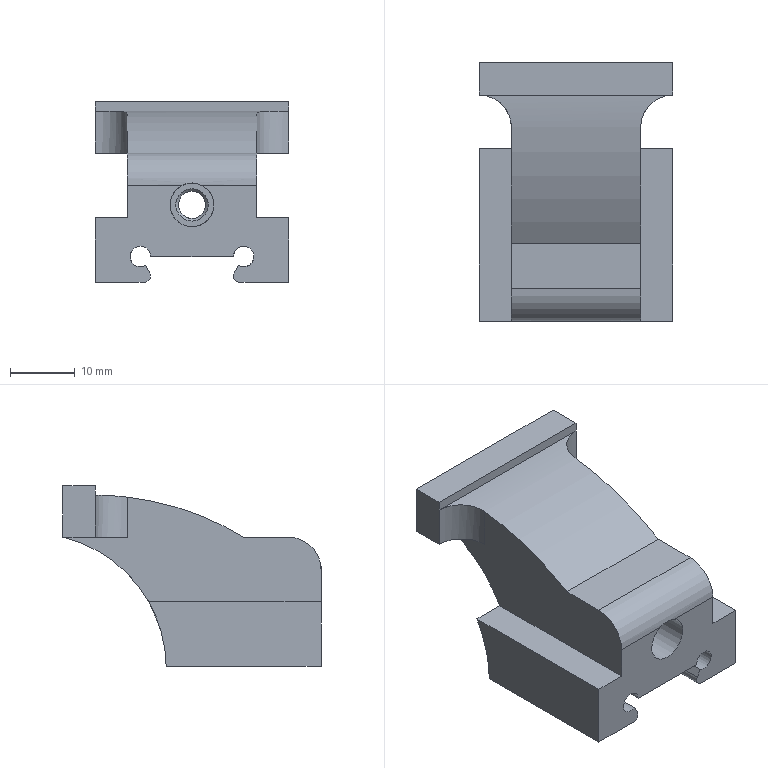Part | NX | features SKETCH 9, EXTRUDE 8, BLEND 3, DATUM_CSYS 1, HOLE PACKAGE 1, SIMPLE HOLE 1, SYMBOLIC_THREAD 1 | 1 solid | 34 faces | box 30 x 40 x 28 mm | volume 14530 mm3 | plane 21 | cylinder 11 | cone 1 | spline 1 | commonest cylinder face diameters 10 x3 2 x2 3.2 x2 4.2 x1 6.8 x1 41.718 x1
STEP:
#1=CARTESIAN_POINT('',(-7.423,0.,-12.));
#2=VERTEX_POINT('',#1);
#3=CARTESIAN_POINT('',(-15.,0.,-12.));
#4=VERTEX_POINT('',#3);
#5=CARTESIAN_POINT('',(15.,0.,-12.));
#6=DIRECTION('',(-1.,0.,0.));
#7=VECTOR('',#6,1000.);
#8=LINE('',#5,#7);
#9=EDGE_CURVE('',#2,#4,#8,.T.);
#10=ORIENTED_EDGE('',*,*,#9,.F.);
#11=CARTESIAN_POINT('',(-6.557,0.,-10.5));
#12=VERTEX_POINT('',#11);
#13=CARTESIAN_POINT('',(-7.423,0.,-11.));
#14=DIRECTION('',(0.,1.,0.));
#15=DIRECTION('',(0.,0.,1.));
#16=AXIS2_PLACEMENT_3D('',#13,#14,#15);
#17=CIRCLE('',#16,1.);
#18=EDGE_CURVE('',#2,#12,#17,.F.);
#19=ORIENTED_EDGE('',*,*,#18,.T.);
#20=CARTESIAN_POINT('',(-7.2,0.,-9.386));
#21=VERTEX_POINT('',#20);
#22=CARTESIAN_POINT('',(-5.691,0.,-12.));
#23=DIRECTION('',(-0.5,0.,0.866));
#24=VECTOR('',#23,1000.);
#25=LINE('',#22,#24);
#26=EDGE_CURVE('',#12,#21,#25,.T.);
#27=ORIENTED_EDGE('',*,*,#26,.T.);
#28=CARTESIAN_POINT('',(-6.4,0.,-8.));
#29=VERTEX_POINT('',#28);
#30=CARTESIAN_POINT('',(-8.,0.,-8.));
#31=DIRECTION('',(0.,1.,0.));
#32=DIRECTION('',(1.,0.,0.));
#33=AXIS2_PLACEMENT_3D('',#30,#31,#32);
#34=CIRCLE('',#33,1.6);
#35=EDGE_CURVE('',#21,#29,#34,.T.);
#36=ORIENTED_EDGE('',*,*,#35,.T.);
#37=CARTESIAN_POINT('',(6.4,0.,-8.));
#38=VERTEX_POINT('',#37);
#39=CARTESIAN_POINT('',(0.,0.,-8.));
#40=DIRECTION('',(1.,0.,0.));
#41=VECTOR('',#40,1000.);
#42=LINE('',#39,#41);
#43=EDGE_CURVE('',#29,#38,#42,.T.);
#44=ORIENTED_EDGE('',*,*,#43,.T.);
#45=CARTESIAN_POINT('',(7.2,0.,-9.386));
#46=VERTEX_POINT('',#45);
#47=CARTESIAN_POINT('',(8.,0.,-8.));
#48=DIRECTION('',(0.,1.,0.));
#49=DIRECTION('',(1.,0.,0.));
#50=AXIS2_PLACEMENT_3D('',#47,#48,#49);
#51=CIRCLE('',#50,1.6);
#52=EDGE_CURVE('',#38,#46,#51,.T.);
#53=ORIENTED_EDGE('',*,*,#52,.T.);
#54=CARTESIAN_POINT('',(6.557,0.,-10.5));
#55=VERTEX_POINT('',#54);
#56=CARTESIAN_POINT('',(7.2,0.,-9.386));
#57=DIRECTION('',(-0.5,0.,-0.866));
#58=VECTOR('',#57,1000.);
#59=LINE('',#56,#58);
#60=EDGE_CURVE('',#46,#55,#59,.T.);
#61=ORIENTED_EDGE('',*,*,#60,.T.);
#62=CARTESIAN_POINT('',(7.423,0.,-12.));
#63=VERTEX_POINT('',#62);
#64=CARTESIAN_POINT('',(7.423,0.,-11.));
#65=DIRECTION('',(0.,1.,0.));
#66=DIRECTION('',(0.,0.,1.));
#67=AXIS2_PLACEMENT_3D('',#64,#65,#66);
#68=CIRCLE('',#67,1.);
#69=EDGE_CURVE('',#55,#63,#68,.F.);
#70=ORIENTED_EDGE('',*,*,#69,.T.);
#71=CARTESIAN_POINT('',(15.,0.,-12.));
#72=VERTEX_POINT('',#71);
#73=CARTESIAN_POINT('',(15.,0.,-12.));
#74=DIRECTION('',(-1.,0.,0.));
#75=VECTOR('',#74,1000.);
#76=LINE('',#73,#75);
#77=EDGE_CURVE('',#72,#63,#76,.T.);
#78=ORIENTED_EDGE('',*,*,#77,.F.);
#79=CARTESIAN_POINT('',(15.,0.,-2.));
#80=VERTEX_POINT('',#79);
#81=CARTESIAN_POINT('',(15.,0.,16.));
#82=DIRECTION('',(0.,0.,-1.));
#83=VECTOR('',#82,1000.);
#84=LINE('',#81,#83);
#85=EDGE_CURVE('',#80,#72,#84,.T.);
#86=ORIENTED_EDGE('',*,*,#85,.F.);
#87=CARTESIAN_POINT('',(10.,0.,-2.));
#88=VERTEX_POINT('',#87);
#89=CARTESIAN_POINT('',(10.,0.,-2.));
#90=DIRECTION('',(1.,0.,0.));
#91=VECTOR('',#90,1000.);
#92=LINE('',#89,#91);
#93=EDGE_CURVE('',#88,#80,#92,.T.);
#94=ORIENTED_EDGE('',*,*,#93,.F.);
#95=CARTESIAN_POINT('',(10.,0.,3.));
#96=VERTEX_POINT('',#95);
#97=CARTESIAN_POINT('',(10.,0.,8.));
#98=DIRECTION('',(0.,0.,-1.));
#99=VECTOR('',#98,1000.);
#100=LINE('',#97,#99);
#101=EDGE_CURVE('',#96,#88,#100,.T.);
#102=ORIENTED_EDGE('',*,*,#101,.F.);
#103=CARTESIAN_POINT('',(1.6,0.,3.));
#104=VERTEX_POINT('',#103);
#105=CARTESIAN_POINT('',(-10.,0.,3.));
#106=DIRECTION('',(1.,0.,0.));
#107=VECTOR('',#106,1000.);
#108=LINE('',#105,#107);
#109=EDGE_CURVE('',#96,#104,#108,.F.);
#110=ORIENTED_EDGE('',*,*,#109,.T.);
#111=CARTESIAN_POINT('',(-1.6,0.,3.));
#112=VERTEX_POINT('',#111);
#113=CARTESIAN_POINT('',(0.,0.,0.));
#114=DIRECTION('',(0.,-1.,0.));
#115=DIRECTION('',(1.,0.,0.));
#116=AXIS2_PLACEMENT_3D('',#113,#114,#115);
#117=CIRCLE('',#116,3.4);
#118=EDGE_CURVE('',#112,#104,#117,.T.);
#119=ORIENTED_EDGE('',*,*,#118,.F.);
#120=CARTESIAN_POINT('',(-10.,0.,3.));
#121=VERTEX_POINT('',#120);
#122=CARTESIAN_POINT('',(-10.,0.,3.));
#123=DIRECTION('',(1.,0.,0.));
#124=VECTOR('',#123,1000.);
#125=LINE('',#122,#124);
#126=EDGE_CURVE('',#112,#121,#125,.F.);
#127=ORIENTED_EDGE('',*,*,#126,.T.);
#128=CARTESIAN_POINT('',(-10.,0.,-2.));
#129=VERTEX_POINT('',#128);
#130=CARTESIAN_POINT('',(-10.,0.,8.));
#131=DIRECTION('',(0.,0.,-1.));
#132=VECTOR('',#131,1000.);
#133=LINE('',#130,#132);
#134=EDGE_CURVE('',#121,#129,#133,.T.);
#135=ORIENTED_EDGE('',*,*,#134,.T.);
#136=CARTESIAN_POINT('',(-15.,0.,-2.));
#137=VERTEX_POINT('',#136);
#138=CARTESIAN_POINT('',(-10.,0.,-2.));
#139=DIRECTION('',(-1.,0.,0.));
#140=VECTOR('',#139,1000.);
#141=LINE('',#138,#140);
#142=EDGE_CURVE('',#129,#137,#141,.T.);
#143=ORIENTED_EDGE('',*,*,#142,.T.);
#144=CARTESIAN_POINT('',(-15.,0.,-12.));
#145=DIRECTION('',(0.,0.,1.));
#146=VECTOR('',#145,1000.);
#147=LINE('',#144,#146);
#148=EDGE_CURVE('',#4,#137,#147,.T.);
#149=ORIENTED_EDGE('',*,*,#148,.F.);
#150=EDGE_LOOP('',(#10,#19,#27,#36,#44,#53,#61,#70,#78,#86,#94,#102,#110,#119,#127,#135,#143,#149));
#151=FACE_BOUND('',#150,.T.);
#152=CARTESIAN_POINT('',(-15.,0.,-12.));
#153=DIRECTION('',(0.,1.,0.));
#154=DIRECTION('',(0.,0.,1.));
#155=AXIS2_PLACEMENT_3D('',#152,#153,#154);
#156=PLANE('',#155);
#157=ADVANCED_FACE('',(#151),#156,.F.);
#158=CARTESIAN_POINT('',(10.,5.,8.));
#159=VERTEX_POINT('',#158);
#160=CARTESIAN_POINT('',(10.,12.,8.));
#161=VERTEX_POINT('',#160);
#162=CARTESIAN_POINT('',(10.,44.,8.));
#163=DIRECTION('',(0.,1.,0.));
#164=VECTOR('',#163,1000.);
#165=LINE('',#162,#164);
#166=EDGE_CURVE('',#159,#161,#165,.T.);
#167=ORIENTED_EDGE('',*,*,#166,.F.);
#168=CARTESIAN_POINT('',(10.,5.,3.));
#169=DIRECTION('',(-1.,0.,0.));
#170=DIRECTION('',(0.,0.,1.));
#171=AXIS2_PLACEMENT_3D('',#168,#169,#170);
#172=CIRCLE('',#171,5.);
#173=EDGE_CURVE('',#159,#96,#172,.F.);
#174=ORIENTED_EDGE('',*,*,#173,.T.);
#175=ORIENTED_EDGE('',*,*,#101,.T.);
#176=CARTESIAN_POINT('',(10.,26.71,-2.));
#177=VERTEX_POINT('',#176);
#178=CARTESIAN_POINT('',(10.,44.,-2.));
#179=DIRECTION('',(0.,-1.,0.));
#180=VECTOR('',#179,1000.);
#181=LINE('',#178,#180);
#182=EDGE_CURVE('',#177,#88,#181,.T.);
#183=ORIENTED_EDGE('',*,*,#182,.F.);
#184=CARTESIAN_POINT('',(10.,40.,8.));
#185=VERTEX_POINT('',#184);
#186=CARTESIAN_POINT('',(10.,44.857,-12.286));
#187=DIRECTION('',(-1.,0.,0.));
#188=DIRECTION('',(0.,0.,1.));
#189=AXIS2_PLACEMENT_3D('',#186,#187,#188);
#190=CIRCLE('',#189,20.859);
#191=EDGE_CURVE('',#185,#177,#190,.F.);
#192=ORIENTED_EDGE('',*,*,#191,.F.);
#193=CARTESIAN_POINT('',(10.,30.,8.));
#194=VERTEX_POINT('',#193);
#195=CARTESIAN_POINT('',(10.,44.,8.));
#196=DIRECTION('',(0.,-1.,0.));
#197=VECTOR('',#196,1000.);
#198=LINE('',#195,#197);
#199=EDGE_CURVE('',#185,#194,#198,.T.);
#200=ORIENTED_EDGE('',*,*,#199,.T.);
#201=CARTESIAN_POINT('',(10.,30.,14.215));
#202=VERTEX_POINT('',#201);
#203=CARTESIAN_POINT('',(10.,30.,16.));
#204=DIRECTION('',(0.,0.,1.));
#205=VECTOR('',#204,1000.);
#206=LINE('',#203,#205);
#207=EDGE_CURVE('',#194,#202,#206,.T.);
#208=ORIENTED_EDGE('',*,*,#207,.T.);
#209=CARTESIAN_POINT('',(10.,35.,-29.442));
#210=DIRECTION('',(-1.,0.,0.));
#211=DIRECTION('',(0.,0.,1.));
#212=AXIS2_PLACEMENT_3D('',#209,#210,#211);
#213=CIRCLE('',#212,43.942);
#214=EDGE_CURVE('',#161,#202,#213,.T.);
#215=ORIENTED_EDGE('',*,*,#214,.F.);
#216=EDGE_LOOP('',(#167,#174,#175,#183,#192,#200,#208,#215));
#217=FACE_BOUND('',#216,.T.);
#218=CARTESIAN_POINT('',(10.,44.,8.));
#219=DIRECTION('',(-1.,0.,0.));
#220=DIRECTION('',(0.,0.,1.));
#221=AXIS2_PLACEMENT_3D('',#218,#219,#220);
#222=PLANE('',#221);
#223=ADVANCED_FACE('',(#217),#222,.F.);
#224=ORIENTED_EDGE('',*,*,#134,.F.);
#225=CARTESIAN_POINT('',(-10.,5.,8.));
#226=VERTEX_POINT('',#225);
#227=CARTESIAN_POINT('',(-10.,5.,3.));
#228=DIRECTION('',(-1.,0.,0.));
#229=DIRECTION('',(0.,0.,1.));
#230=AXIS2_PLACEMENT_3D('',#227,#228,#229);
#231=CIRCLE('',#230,5.);
#232=EDGE_CURVE('',#121,#226,#231,.T.);
#233=ORIENTED_EDGE('',*,*,#232,.T.);
#234=CARTESIAN_POINT('',(-10.,12.,8.));
#235=VERTEX_POINT('',#234);
#236=CARTESIAN_POINT('',(-10.,44.,8.));
#237=DIRECTION('',(0.,1.,0.));
#238=VECTOR('',#237,1000.);
#239=LINE('',#236,#238);
#240=EDGE_CURVE('',#226,#235,#239,.T.);
#241=ORIENTED_EDGE('',*,*,#240,.T.);
#242=CARTESIAN_POINT('',(-10.,30.,14.215));
#243=VERTEX_POINT('',#242);
#244=CARTESIAN_POINT('',(-10.,35.,-29.442));
#245=DIRECTION('',(-1.,0.,0.));
#246=DIRECTION('',(0.,0.,1.));
#247=AXIS2_PLACEMENT_3D('',#244,#245,#246);
#248=CIRCLE('',#247,43.942);
#249=EDGE_CURVE('',#235,#243,#248,.T.);
#250=ORIENTED_EDGE('',*,*,#249,.T.);
#251=CARTESIAN_POINT('',(-10.,30.,8.));
#252=VERTEX_POINT('',#251);
#253=CARTESIAN_POINT('',(-10.,30.,8.));
#254=DIRECTION('',(0.,0.,1.));
#255=VECTOR('',#254,1000.);
#256=LINE('',#253,#255);
#257=EDGE_CURVE('',#243,#252,#256,.F.);
#258=ORIENTED_EDGE('',*,*,#257,.T.);
#259=CARTESIAN_POINT('',(-10.,40.,8.));
#260=VERTEX_POINT('',#259);
#261=CARTESIAN_POINT('',(-10.,44.,8.));
#262=DIRECTION('',(0.,-1.,0.));
#263=VECTOR('',#262,1000.);
#264=LINE('',#261,#263);
#265=EDGE_CURVE('',#260,#252,#264,.T.);
#266=ORIENTED_EDGE('',*,*,#265,.F.);
#267=CARTESIAN_POINT('',(-10.,26.71,-2.));
#268=VERTEX_POINT('',#267);
#269=CARTESIAN_POINT('',(-10.,44.857,-12.286));
#270=DIRECTION('',(-1.,0.,0.));
#271=DIRECTION('',(0.,0.,1.));
#272=AXIS2_PLACEMENT_3D('',#269,#270,#271);
#273=CIRCLE('',#272,20.859);
#274=EDGE_CURVE('',#260,#268,#273,.F.);
#275=ORIENTED_EDGE('',*,*,#274,.T.);
#276=CARTESIAN_POINT('',(-10.,44.,-2.));
#277=DIRECTION('',(0.,-1.,0.));
#278=VECTOR('',#277,1000.);
#279=LINE('',#276,#278);
#280=EDGE_CURVE('',#268,#129,#279,.T.);
#281=ORIENTED_EDGE('',*,*,#280,.T.);
#282=EDGE_LOOP('',(#224,#233,#241,#250,#258,#266,#275,#281));
#283=FACE_BOUND('',#282,.T.);
#284=CARTESIAN_POINT('',(-10.,44.,8.));
#285=DIRECTION('',(-1.,0.,0.));
#286=DIRECTION('',(0.,0.,1.));
#287=AXIS2_PLACEMENT_3D('',#284,#285,#286);
#288=PLANE('',#287);
#289=ADVANCED_FACE('',(#283),#288,.T.);
#290=CARTESIAN_POINT('',(-15.,35.,14.5));
#291=VERTEX_POINT('',#290);
#292=CARTESIAN_POINT('',(-15.,35.,14.5));
#293=CARTESIAN_POINT('',(-13.678,35.,14.5));
#294=CARTESIAN_POINT('',(-11.086,33.91,14.519));
#295=CARTESIAN_POINT('',(-10.,31.314,14.365));
#296=CARTESIAN_POINT('',(-10.,30.,14.215));
#297=B_SPLINE_CURVE_WITH_KNOTS('',3,(#292,#293,#294,#295,#296),.UNSPECIFIED.,.F.,.F.,(4,1,4),(0.,0.003911,0.007821),.UNSPECIFIED.);
#298=EDGE_CURVE('',#291,#243,#297,.T.);
#299=ORIENTED_EDGE('',*,*,#298,.F.);
#300=CARTESIAN_POINT('',(-15.,35.,8.));
#301=VERTEX_POINT('',#300);
#302=CARTESIAN_POINT('',(-15.,35.,-12.));
#303=DIRECTION('',(0.,0.,-1.));
#304=VECTOR('',#303,1000.);
#305=LINE('',#302,#304);
#306=EDGE_CURVE('',#291,#301,#305,.T.);
#307=ORIENTED_EDGE('',*,*,#306,.T.);
#308=CARTESIAN_POINT('',(-15.,30.,8.));
#309=DIRECTION('',(0.,0.,-1.));
#310=DIRECTION('',(-1.,0.,0.));
#311=AXIS2_PLACEMENT_3D('',#308,#309,#310);
#312=CIRCLE('',#311,5.);
#313=EDGE_CURVE('',#252,#301,#312,.F.);
#314=ORIENTED_EDGE('',*,*,#313,.F.);
#315=ORIENTED_EDGE('',*,*,#257,.F.);
#316=EDGE_LOOP('',(#299,#307,#314,#315));
#317=FACE_BOUND('',#316,.T.);
#318=CARTESIAN_POINT('',(-15.,30.,-162.2));
#319=DIRECTION('',(0.,0.,-1.));
#320=DIRECTION('',(-1.,0.,0.));
#321=AXIS2_PLACEMENT_3D('',#318,#319,#320);
#322=CYLINDRICAL_SURFACE('',#321,5.);
#323=ADVANCED_FACE('',(#317),#322,.F.);
#324=CARTESIAN_POINT('',(15.,35.,14.5));
#325=VERTEX_POINT('',#324);
#326=CARTESIAN_POINT('',(10.,30.,14.215));
#327=CARTESIAN_POINT('',(10.,31.314,14.365));
#328=CARTESIAN_POINT('',(11.08,33.905,14.518));
#329=CARTESIAN_POINT('',(13.678,35.,14.5));
#330=CARTESIAN_POINT('',(15.,35.,14.5));
#331=B_SPLINE_CURVE_WITH_KNOTS('',3,(#326,#327,#328,#329,#330),.UNSPECIFIED.,.F.,.F.,(4,1,4),(0.,0.003911,0.007821),.UNSPECIFIED.);
#332=EDGE_CURVE('',#202,#325,#331,.T.);
#333=ORIENTED_EDGE('',*,*,#332,.F.);
#334=ORIENTED_EDGE('',*,*,#207,.F.);
#335=CARTESIAN_POINT('',(15.,35.,8.));
#336=VERTEX_POINT('',#335);
#337=CARTESIAN_POINT('',(15.,30.,8.));
#338=DIRECTION('',(0.,0.,1.));
#339=DIRECTION('',(1.,0.,0.));
#340=AXIS2_PLACEMENT_3D('',#337,#338,#339);
#341=CIRCLE('',#340,5.);
#342=EDGE_CURVE('',#336,#194,#341,.T.);
#343=ORIENTED_EDGE('',*,*,#342,.F.);
#344=CARTESIAN_POINT('',(15.,35.,16.));
#345=DIRECTION('',(0.,0.,-1.));
#346=VECTOR('',#345,1000.);
#347=LINE('',#344,#346);
#348=EDGE_CURVE('',#325,#336,#347,.T.);
#349=ORIENTED_EDGE('',*,*,#348,.F.);
#350=EDGE_LOOP('',(#333,#334,#343,#349));
#351=FACE_BOUND('',#350,.T.);
#352=CARTESIAN_POINT('',(15.,30.,8.));
#353=DIRECTION('',(0.,0.,-1.));
#354=DIRECTION('',(-1.,0.,0.));
#355=AXIS2_PLACEMENT_3D('',#352,#353,#354);
#356=CYLINDRICAL_SURFACE('',#355,5.);
#357=ADVANCED_FACE('',(#351),#356,.F.);
#358=CARTESIAN_POINT('',(15.,35.,16.));
#359=VERTEX_POINT('',#358);
#360=CARTESIAN_POINT('',(-15.,35.,16.));
#361=VERTEX_POINT('',#360);
#362=CARTESIAN_POINT('',(0.,35.,16.));
#363=DIRECTION('',(-1.,0.,0.));
#364=VECTOR('',#363,1000.);
#365=LINE('',#362,#364);
#366=EDGE_CURVE('',#359,#361,#365,.T.);
#367=ORIENTED_EDGE('',*,*,#366,.F.);
#368=CARTESIAN_POINT('',(15.,40.,16.));
#369=VERTEX_POINT('',#368);
#370=CARTESIAN_POINT('',(15.,40.,16.));
#371=DIRECTION('',(0.,-1.,0.));
#372=VECTOR('',#371,1000.);
#373=LINE('',#370,#372);
#374=EDGE_CURVE('',#369,#359,#373,.T.);
#375=ORIENTED_EDGE('',*,*,#374,.F.);
#376=CARTESIAN_POINT('',(-15.,40.,16.));
#377=VERTEX_POINT('',#376);
#378=CARTESIAN_POINT('',(-15.,40.,16.));
#379=DIRECTION('',(1.,0.,0.));
#380=VECTOR('',#379,1000.);
#381=LINE('',#378,#380);
#382=EDGE_CURVE('',#377,#369,#381,.T.);
#383=ORIENTED_EDGE('',*,*,#382,.F.);
#384=CARTESIAN_POINT('',(-15.,40.,16.));
#385=DIRECTION('',(0.,-1.,0.));
#386=VECTOR('',#385,1000.);
#387=LINE('',#384,#386);
#388=EDGE_CURVE('',#377,#361,#387,.T.);
#389=ORIENTED_EDGE('',*,*,#388,.T.);
#390=EDGE_LOOP('',(#367,#375,#383,#389));
#391=FACE_BOUND('',#390,.T.);
#392=CARTESIAN_POINT('',(0.,40.,16.));
#393=DIRECTION('',(0.,0.,-1.));
#394=DIRECTION('',(-1.,0.,0.));
#395=AXIS2_PLACEMENT_3D('',#392,#393,#394);
#396=PLANE('',#395);
#397=ADVANCED_FACE('',(#391),#396,.F.);
#398=CARTESIAN_POINT('',(-15.,35.,-12.));
#399=DIRECTION('',(0.,0.,-1.));
#400=VECTOR('',#399,1000.);
#401=LINE('',#398,#400);
#402=EDGE_CURVE('',#361,#291,#401,.T.);
#403=ORIENTED_EDGE('',*,*,#402,.F.);
#404=ORIENTED_EDGE('',*,*,#388,.F.);
#405=CARTESIAN_POINT('',(-15.,40.,8.));
#406=VERTEX_POINT('',#405);
#407=CARTESIAN_POINT('',(-15.,40.,-12.));
#408=DIRECTION('',(0.,0.,1.));
#409=VECTOR('',#408,1000.);
#410=LINE('',#407,#409);
#411=EDGE_CURVE('',#406,#377,#410,.T.);
#412=ORIENTED_EDGE('',*,*,#411,.F.);
#413=CARTESIAN_POINT('',(-15.,40.,8.));
#414=DIRECTION('',(0.,1.,0.));
#415=VECTOR('',#414,1000.);
#416=LINE('',#413,#415);
#417=EDGE_CURVE('',#301,#406,#416,.T.);
#418=ORIENTED_EDGE('',*,*,#417,.F.);
#419=ORIENTED_EDGE('',*,*,#306,.F.);
#420=EDGE_LOOP('',(#403,#404,#412,#418,#419));
#421=FACE_BOUND('',#420,.T.);
#422=CARTESIAN_POINT('',(-15.,40.,-12.));
#423=DIRECTION('',(1.,0.,0.));
#424=DIRECTION('',(0.,0.,-1.));
#425=AXIS2_PLACEMENT_3D('',#422,#423,#424);
#426=PLANE('',#425);
#427=ADVANCED_FACE('',(#421),#426,.F.);
#428=ORIENTED_EDGE('',*,*,#265,.T.);
#429=ORIENTED_EDGE('',*,*,#313,.T.);
#430=ORIENTED_EDGE('',*,*,#417,.T.);
#431=CARTESIAN_POINT('',(-15.,40.,8.));
#432=DIRECTION('',(-1.,0.,0.));
#433=VECTOR('',#432,1000.);
#434=LINE('',#431,#433);
#435=EDGE_CURVE('',#260,#406,#434,.T.);
#436=ORIENTED_EDGE('',*,*,#435,.F.);
#437=EDGE_LOOP('',(#428,#429,#430,#436));
#438=FACE_BOUND('',#437,.T.);
#439=CARTESIAN_POINT('',(-26.,44.,8.));
#440=DIRECTION('',(0.,0.,-1.));
#441=DIRECTION('',(-1.,0.,0.));
#442=AXIS2_PLACEMENT_3D('',#439,#440,#441);
#443=PLANE('',#442);
#444=ADVANCED_FACE('',(#438),#443,.T.);
#445=CARTESIAN_POINT('',(15.,40.,8.));
#446=VERTEX_POINT('',#445);
#447=CARTESIAN_POINT('',(-15.,40.,8.));
#448=DIRECTION('',(1.,0.,0.));
#449=VECTOR('',#448,1000.);
#450=LINE('',#447,#449);
#451=EDGE_CURVE('',#185,#446,#450,.T.);
#452=ORIENTED_EDGE('',*,*,#451,.F.);
#453=CARTESIAN_POINT('',(-18.,40.,8.));
#454=DIRECTION('',(1.,0.,0.));
#455=VECTOR('',#454,1000.);
#456=LINE('',#453,#455);
#457=EDGE_CURVE('',#260,#185,#456,.T.);
#458=ORIENTED_EDGE('',*,*,#457,.F.);
#459=ORIENTED_EDGE('',*,*,#435,.T.);
#460=ORIENTED_EDGE('',*,*,#411,.T.);
#461=ORIENTED_EDGE('',*,*,#382,.T.);
#462=CARTESIAN_POINT('',(15.,40.,16.));
#463=DIRECTION('',(0.,0.,-1.));
#464=VECTOR('',#463,1000.);
#465=LINE('',#462,#464);
#466=EDGE_CURVE('',#369,#446,#465,.T.);
#467=ORIENTED_EDGE('',*,*,#466,.T.);
#468=EDGE_LOOP('',(#452,#458,#459,#460,#461,#467));
#469=FACE_BOUND('',#468,.T.);
#470=CARTESIAN_POINT('',(-15.,40.,-12.));
#471=DIRECTION('',(0.,1.,0.));
#472=DIRECTION('',(0.,0.,1.));
#473=AXIS2_PLACEMENT_3D('',#470,#471,#472);
#474=PLANE('',#473);
#475=ADVANCED_FACE('',(#469),#474,.T.);
#476=CARTESIAN_POINT('',(-15.,24.,-12.));
#477=VERTEX_POINT('',#476);
#478=CARTESIAN_POINT('',(-7.423,24.,-12.));
#479=VERTEX_POINT('',#478);
#480=CARTESIAN_POINT('',(-18.,24.,-12.));
#481=DIRECTION('',(1.,0.,0.));
#482=VECTOR('',#481,1000.);
#483=LINE('',#480,#482);
#484=EDGE_CURVE('',#477,#479,#483,.T.);
#485=ORIENTED_EDGE('',*,*,#484,.T.);
#486=CARTESIAN_POINT('',(-7.423,0.,-12.));
#487=DIRECTION('',(0.,-1.,0.));
#488=VECTOR('',#487,1000.);
#489=LINE('',#486,#488);
#490=EDGE_CURVE('',#479,#2,#489,.T.);
#491=ORIENTED_EDGE('',*,*,#490,.T.);
#492=ORIENTED_EDGE('',*,*,#9,.T.);
#493=CARTESIAN_POINT('',(-15.,40.,-12.));
#494=DIRECTION('',(0.,-1.,0.));
#495=VECTOR('',#494,1000.);
#496=LINE('',#493,#495);
#497=EDGE_CURVE('',#477,#4,#496,.T.);
#498=ORIENTED_EDGE('',*,*,#497,.F.);
#499=EDGE_LOOP('',(#485,#491,#492,#498));
#500=FACE_BOUND('',#499,.T.);
#501=CARTESIAN_POINT('',(15.,40.,-12.));
#502=DIRECTION('',(0.,0.,1.));
#503=DIRECTION('',(1.,0.,0.));
#504=AXIS2_PLACEMENT_3D('',#501,#502,#503);
#505=PLANE('',#504);
#506=ADVANCED_FACE('',(#500),#505,.F.);
#507=ORIENTED_EDGE('',*,*,#77,.T.);
#508=CARTESIAN_POINT('',(7.423,24.,-12.));
#509=VERTEX_POINT('',#508);
#510=CARTESIAN_POINT('',(7.423,24.,-12.));
#511=DIRECTION('',(0.,-1.,0.));
#512=VECTOR('',#511,1000.);
#513=LINE('',#510,#512);
#514=EDGE_CURVE('',#63,#509,#513,.F.);
#515=ORIENTED_EDGE('',*,*,#514,.T.);
#516=CARTESIAN_POINT('',(15.,24.,-12.));
#517=VERTEX_POINT('',#516);
#518=CARTESIAN_POINT('',(-18.,24.,-12.));
#519=DIRECTION('',(1.,0.,0.));
#520=VECTOR('',#519,1000.);
#521=LINE('',#518,#520);
#522=EDGE_CURVE('',#509,#517,#521,.T.);
#523=ORIENTED_EDGE('',*,*,#522,.T.);
#524=CARTESIAN_POINT('',(15.,40.,-12.));
#525=DIRECTION('',(0.,-1.,0.));
#526=VECTOR('',#525,1000.);
#527=LINE('',#524,#526);
#528=EDGE_CURVE('',#517,#72,#527,.T.);
#529=ORIENTED_EDGE('',*,*,#528,.T.);
#530=EDGE_LOOP('',(#507,#515,#523,#529));
#531=FACE_BOUND('',#530,.T.);
#532=CARTESIAN_POINT('',(15.,40.,-12.));
#533=DIRECTION('',(0.,0.,1.));
#534=DIRECTION('',(1.,0.,0.));
#535=AXIS2_PLACEMENT_3D('',#532,#533,#534);
#536=PLANE('',#535);
#537=ADVANCED_FACE('',(#531),#536,.F.);
#538=CARTESIAN_POINT('',(-15.,26.71,-2.));
#539=VERTEX_POINT('',#538);
#540=CARTESIAN_POINT('',(-15.,44.857,-12.286));
#541=DIRECTION('',(1.,0.,0.));
#542=DIRECTION('',(0.,0.,-1.));
#543=AXIS2_PLACEMENT_3D('',#540,#541,#542);
#544=CIRCLE('',#543,20.859);
#545=EDGE_CURVE('',#477,#539,#544,.F.);
#546=ORIENTED_EDGE('',*,*,#545,.F.);
#547=ORIENTED_EDGE('',*,*,#497,.T.);
#548=ORIENTED_EDGE('',*,*,#148,.T.);
#549=CARTESIAN_POINT('',(-15.,40.,-2.));
#550=DIRECTION('',(0.,-1.,0.));
#551=VECTOR('',#550,1000.);
#552=LINE('',#549,#551);
#553=EDGE_CURVE('',#539,#137,#552,.T.);
#554=ORIENTED_EDGE('',*,*,#553,.F.);
#555=EDGE_LOOP('',(#546,#547,#548,#554));
#556=FACE_BOUND('',#555,.T.);
#557=CARTESIAN_POINT('',(-15.,40.,-12.));
#558=DIRECTION('',(1.,0.,0.));
#559=DIRECTION('',(0.,0.,-1.));
#560=AXIS2_PLACEMENT_3D('',#557,#558,#559);
#561=PLANE('',#560);
#562=ADVANCED_FACE('',(#556),#561,.F.);
#563=CARTESIAN_POINT('',(15.,26.71,-2.));
#564=VERTEX_POINT('',#563);
#565=CARTESIAN_POINT('',(15.,44.857,-12.286));
#566=DIRECTION('',(-1.,0.,0.));
#567=DIRECTION('',(0.,1.,0.));
#568=AXIS2_PLACEMENT_3D('',#565,#566,#567);
#569=CIRCLE('',#568,20.859);
#570=EDGE_CURVE('',#517,#564,#569,.T.);
#571=ORIENTED_EDGE('',*,*,#570,.T.);
#572=CARTESIAN_POINT('',(15.,40.,-2.));
#573=DIRECTION('',(0.,-1.,0.));
#574=VECTOR('',#573,1000.);
#575=LINE('',#572,#574);
#576=EDGE_CURVE('',#564,#80,#575,.T.);
#577=ORIENTED_EDGE('',*,*,#576,.T.);
#578=ORIENTED_EDGE('',*,*,#85,.T.);
#579=ORIENTED_EDGE('',*,*,#528,.F.);
#580=EDGE_LOOP('',(#571,#577,#578,#579));
#581=FACE_BOUND('',#580,.T.);
#582=CARTESIAN_POINT('',(15.,40.,16.));
#583=DIRECTION('',(-1.,0.,0.));
#584=DIRECTION('',(0.,0.,1.));
#585=AXIS2_PLACEMENT_3D('',#582,#583,#584);
#586=PLANE('',#585);
#587=ADVANCED_FACE('',(#581),#586,.F.);
#588=CARTESIAN_POINT('',(-18.,26.71,-2.));
#589=DIRECTION('',(1.,0.,0.));
#590=VECTOR('',#589,1000.);
#591=LINE('',#588,#590);
#592=EDGE_CURVE('',#177,#564,#591,.T.);
#593=ORIENTED_EDGE('',*,*,#592,.F.);
#594=ORIENTED_EDGE('',*,*,#182,.T.);
#595=ORIENTED_EDGE('',*,*,#93,.T.);
#596=ORIENTED_EDGE('',*,*,#576,.F.);
#597=EDGE_LOOP('',(#593,#594,#595,#596));
#598=FACE_BOUND('',#597,.T.);
#599=CARTESIAN_POINT('',(10.,44.,-2.));
#600=DIRECTION('',(0.,0.,-1.));
#601=DIRECTION('',(-1.,0.,0.));
#602=AXIS2_PLACEMENT_3D('',#599,#600,#601);
#603=PLANE('',#602);
#604=ADVANCED_FACE('',(#598),#603,.F.);
#605=ORIENTED_EDGE('',*,*,#280,.F.);
#606=CARTESIAN_POINT('',(-18.,26.71,-2.));
#607=DIRECTION('',(1.,0.,0.));
#608=VECTOR('',#607,1000.);
#609=LINE('',#606,#608);
#610=EDGE_CURVE('',#268,#539,#609,.F.);
#611=ORIENTED_EDGE('',*,*,#610,.T.);
#612=ORIENTED_EDGE('',*,*,#553,.T.);
#613=ORIENTED_EDGE('',*,*,#142,.F.);
#614=EDGE_LOOP('',(#605,#611,#612,#613));
#615=FACE_BOUND('',#614,.T.);
#616=CARTESIAN_POINT('',(-10.,44.,-2.));
#617=DIRECTION('',(0.,0.,1.));
#618=DIRECTION('',(1.,0.,0.));
#619=AXIS2_PLACEMENT_3D('',#616,#617,#618);
#620=PLANE('',#619);
#621=ADVANCED_FACE('',(#615),#620,.T.);
#622=ORIENTED_EDGE('',*,*,#26,.F.);
#623=CARTESIAN_POINT('',(-6.557,24.075,-10.5));
#624=VERTEX_POINT('',#623);
#625=CARTESIAN_POINT('',(-6.557,24.,-10.5));
#626=DIRECTION('',(0.,-1.,0.));
#627=VECTOR('',#626,1000.);
#628=LINE('',#625,#627);
#629=EDGE_CURVE('',#12,#624,#628,.F.);
#630=ORIENTED_EDGE('',*,*,#629,.T.);
#631=CARTESIAN_POINT('',(-7.2,24.201,-9.386));
#632=VERTEX_POINT('',#631);
#633=CARTESIAN_POINT('',(-5.526,44.857,-12.286));
#634=DIRECTION('',(0.866,0.,0.5));
#635=DIRECTION('',(0.5,0.,-0.866));
#636=AXIS2_PLACEMENT_3D('',#633,#634,#635);
#637=ELLIPSE('',#636,24.086,20.859);
#638=EDGE_CURVE('',#624,#632,#637,.F.);
#639=ORIENTED_EDGE('',*,*,#638,.T.);
#640=CARTESIAN_POINT('',(-7.2,44.,-9.386));
#641=DIRECTION('',(0.,-1.,0.));
#642=VECTOR('',#641,1000.);
#643=LINE('',#640,#642);
#644=EDGE_CURVE('',#632,#21,#643,.T.);
#645=ORIENTED_EDGE('',*,*,#644,.T.);
#646=EDGE_LOOP('',(#622,#630,#639,#645));
#647=FACE_BOUND('',#646,.T.);
#648=CARTESIAN_POINT('',(-5.691,44.,-12.));
#649=DIRECTION('',(0.866,0.,0.5));
#650=DIRECTION('',(0.5,0.,-0.866));
#651=AXIS2_PLACEMENT_3D('',#648,#649,#650);
#652=PLANE('',#651);
#653=ADVANCED_FACE('',(#647),#652,.T.);
#654=ORIENTED_EDGE('',*,*,#644,.F.);
#655=CARTESIAN_POINT('',(-6.4,24.443,-8.));
#656=VERTEX_POINT('',#655);
#657=CARTESIAN_POINT('',(-7.2,24.201,-9.386));
#658=CARTESIAN_POINT('',(-7.816,24.151,-9.741));
#659=CARTESIAN_POINT('',(-9.524,24.164,-9.466));
#660=CARTESIAN_POINT('',(-9.768,24.562,-7.377));
#661=CARTESIAN_POINT('',(-8.661,24.842,-6.413));
#662=CARTESIAN_POINT('',(-7.159,24.869,-6.315));
#663=CARTESIAN_POINT('',(-6.4,24.589,-7.303));
#664=CARTESIAN_POINT('',(-6.4,24.443,-8.));
#665=B_SPLINE_CURVE_WITH_KNOTS('',3,(#657,#658,#659,#660,#661,#662,#663,#664),.UNSPECIFIED.,.F.,.F.,(4,1,1,1,1,4),(0.,0.002108,0.004216,0.00527,0.006324,0.008432),.UNSPECIFIED.);
#666=EDGE_CURVE('',#632,#656,#665,.T.);
#667=ORIENTED_EDGE('',*,*,#666,.T.);
#668=CARTESIAN_POINT('',(-6.4,44.,-8.));
#669=DIRECTION('',(0.,-1.,0.));
#670=VECTOR('',#669,1000.);
#671=LINE('',#668,#670);
#672=EDGE_CURVE('',#656,#29,#671,.T.);
#673=ORIENTED_EDGE('',*,*,#672,.T.);
#674=ORIENTED_EDGE('',*,*,#35,.F.);
#675=EDGE_LOOP('',(#654,#667,#673,#674));
#676=FACE_BOUND('',#675,.T.);
#677=CARTESIAN_POINT('',(-8.,44.,-8.));
#678=DIRECTION('',(0.,-1.,0.));
#679=DIRECTION('',(0.,0.,-1.));
#680=AXIS2_PLACEMENT_3D('',#677,#678,#679);
#681=CYLINDRICAL_SURFACE('',#680,1.6);
#682=ADVANCED_FACE('',(#676),#681,.F.);
#683=ORIENTED_EDGE('',*,*,#672,.F.);
#684=CARTESIAN_POINT('',(6.4,24.443,-8.));
#685=VERTEX_POINT('',#684);
#686=CARTESIAN_POINT('',(-18.,24.443,-8.));
#687=DIRECTION('',(1.,0.,0.));
#688=VECTOR('',#687,1000.);
#689=LINE('',#686,#688);
#690=EDGE_CURVE('',#656,#685,#689,.T.);
#691=ORIENTED_EDGE('',*,*,#690,.T.);
#692=CARTESIAN_POINT('',(6.4,44.,-8.));
#693=DIRECTION('',(0.,-1.,0.));
#694=VECTOR('',#693,1000.);
#695=LINE('',#692,#694);
#696=EDGE_CURVE('',#685,#38,#695,.T.);
#697=ORIENTED_EDGE('',*,*,#696,.T.);
#698=ORIENTED_EDGE('',*,*,#43,.F.);
#699=EDGE_LOOP('',(#683,#691,#697,#698));
#700=FACE_BOUND('',#699,.T.);
#701=CARTESIAN_POINT('',(0.,44.,-8.));
#702=DIRECTION('',(0.,0.,-1.));
#703=DIRECTION('',(-1.,0.,0.));
#704=AXIS2_PLACEMENT_3D('',#701,#702,#703);
#705=PLANE('',#704);
#706=ADVANCED_FACE('',(#700),#705,.T.);
#707=ORIENTED_EDGE('',*,*,#696,.F.);
#708=CARTESIAN_POINT('',(7.2,24.201,-9.386));
#709=VERTEX_POINT('',#708);
#710=CARTESIAN_POINT('',(6.4,24.443,-8.));
#711=CARTESIAN_POINT('',(6.4,24.589,-7.303));
#712=CARTESIAN_POINT('',(7.154,24.868,-6.318));
#713=CARTESIAN_POINT('',(8.657,24.843,-6.411));
#714=CARTESIAN_POINT('',(9.768,24.563,-7.374));
#715=CARTESIAN_POINT('',(9.527,24.164,-9.464));
#716=CARTESIAN_POINT('',(7.816,24.151,-9.741));
#717=CARTESIAN_POINT('',(7.2,24.201,-9.386));
#718=B_SPLINE_CURVE_WITH_KNOTS('',3,(#710,#711,#712,#713,#714,#715,#716,#717),.UNSPECIFIED.,.F.,.F.,(4,1,1,1,1,4),(0.,0.002107,0.003161,0.004214,0.006321,0.008428),.UNSPECIFIED.);
#719=EDGE_CURVE('',#685,#709,#718,.T.);
#720=ORIENTED_EDGE('',*,*,#719,.T.);
#721=CARTESIAN_POINT('',(7.2,44.,-9.386));
#722=DIRECTION('',(0.,-1.,0.));
#723=VECTOR('',#722,1000.);
#724=LINE('',#721,#723);
#725=EDGE_CURVE('',#709,#46,#724,.T.);
#726=ORIENTED_EDGE('',*,*,#725,.T.);
#727=ORIENTED_EDGE('',*,*,#52,.F.);
#728=EDGE_LOOP('',(#707,#720,#726,#727));
#729=FACE_BOUND('',#728,.T.);
#730=CARTESIAN_POINT('',(8.,44.,-8.));
#731=DIRECTION('',(0.,-1.,0.));
#732=DIRECTION('',(0.,0.,-1.));
#733=AXIS2_PLACEMENT_3D('',#730,#731,#732);
#734=CYLINDRICAL_SURFACE('',#733,1.6);
#735=ADVANCED_FACE('',(#729),#734,.F.);
#736=CARTESIAN_POINT('',(6.557,24.075,-10.5));
#737=VERTEX_POINT('',#736);
#738=CARTESIAN_POINT('',(5.526,44.857,-12.286));
#739=DIRECTION('',(-0.866,0.,0.5));
#740=DIRECTION('',(0.5,0.,0.866));
#741=AXIS2_PLACEMENT_3D('',#738,#739,#740);
#742=ELLIPSE('',#741,24.086,20.859);
#743=EDGE_CURVE('',#709,#737,#742,.F.);
#744=ORIENTED_EDGE('',*,*,#743,.T.);
#745=CARTESIAN_POINT('',(6.557,0.,-10.5));
#746=DIRECTION('',(0.,-1.,0.));
#747=VECTOR('',#746,1000.);
#748=LINE('',#745,#747);
#749=EDGE_CURVE('',#737,#55,#748,.T.);
#750=ORIENTED_EDGE('',*,*,#749,.T.);
#751=ORIENTED_EDGE('',*,*,#60,.F.);
#752=ORIENTED_EDGE('',*,*,#725,.F.);
#753=EDGE_LOOP('',(#744,#750,#751,#752));
#754=FACE_BOUND('',#753,.T.);
#755=CARTESIAN_POINT('',(7.2,44.,-9.386));
#756=DIRECTION('',(-0.866,0.,0.5));
#757=DIRECTION('',(0.5,0.,0.866));
#758=AXIS2_PLACEMENT_3D('',#755,#756,#757);
#759=PLANE('',#758);
#760=ADVANCED_FACE('',(#754),#759,.T.);
#761=ORIENTED_EDGE('',*,*,#374,.T.);
#762=CARTESIAN_POINT('',(15.,35.,16.));
#763=DIRECTION('',(0.,0.,-1.));
#764=VECTOR('',#763,1000.);
#765=LINE('',#762,#764);
#766=EDGE_CURVE('',#359,#325,#765,.T.);
#767=ORIENTED_EDGE('',*,*,#766,.T.);
#768=ORIENTED_EDGE('',*,*,#348,.T.);
#769=CARTESIAN_POINT('',(15.,40.,8.));
#770=DIRECTION('',(0.,1.,0.));
#771=VECTOR('',#770,1000.);
#772=LINE('',#769,#771);
#773=EDGE_CURVE('',#336,#446,#772,.T.);
#774=ORIENTED_EDGE('',*,*,#773,.T.);
#775=ORIENTED_EDGE('',*,*,#466,.F.);
#776=EDGE_LOOP('',(#761,#767,#768,#774,#775));
#777=FACE_BOUND('',#776,.T.);
#778=CARTESIAN_POINT('',(15.,40.,16.));
#779=DIRECTION('',(-1.,0.,0.));
#780=DIRECTION('',(0.,0.,1.));
#781=AXIS2_PLACEMENT_3D('',#778,#779,#780);
#782=PLANE('',#781);
#783=ADVANCED_FACE('',(#777),#782,.F.);
#784=ORIENTED_EDGE('',*,*,#773,.F.);
#785=ORIENTED_EDGE('',*,*,#342,.T.);
#786=ORIENTED_EDGE('',*,*,#199,.F.);
#787=ORIENTED_EDGE('',*,*,#451,.T.);
#788=EDGE_LOOP('',(#784,#785,#786,#787));
#789=FACE_BOUND('',#788,.T.);
#790=CARTESIAN_POINT('',(26.,44.,8.));
#791=DIRECTION('',(0.,0.,1.));
#792=DIRECTION('',(1.,0.,0.));
#793=AXIS2_PLACEMENT_3D('',#790,#791,#792);
#794=PLANE('',#793);
#795=ADVANCED_FACE('',(#789),#794,.F.);
#796=CARTESIAN_POINT('',(0.,29.868,2.221));
#797=VERTEX_POINT('',#796);
#798=CARTESIAN_POINT('',(1.145,29.685,2.034));
#799=CARTESIAN_POINT('',(0.03763,29.95,2.304));
#800=CARTESIAN_POINT('',(-1.048,29.718,2.067));
#801=CARTESIAN_POINT('',(-2.099,29.032,1.325));
#802=CARTESIAN_POINT('',(-2.577,28.17,0.2701));
#803=CARTESIAN_POINT('',(-2.455,27.318,-0.9777));
#804=CARTESIAN_POINT('',(-2.014,26.819,-1.798));
#805=CARTESIAN_POINT('',(-1.181,26.439,-2.489));
#806=CARTESIAN_POINT('',(-0.07159,26.294,-2.772));
#807=CARTESIAN_POINT('',(1.03,26.406,-2.552));
#808=CARTESIAN_POINT('',(2.189,26.851,-1.729));
#809=CARTESIAN_POINT('',(2.71,27.806,-0.1994));
#810=CARTESIAN_POINT('',(2.19,28.929,1.208));
#811=CARTESIAN_POINT('',(1.145,29.685,2.034));
#812=CARTESIAN_POINT('',(0.03763,29.95,2.304));
#813=CARTESIAN_POINT('',(-1.048,29.718,2.067));
#814=B_SPLINE_CURVE_WITH_KNOTS('',3,(#798,#799,#800,#801,#802,#803,#804,#805,#806,#807,#808,#809,#810,#811,#812,#813),.UNSPECIFIED.,.T.,.F.,(1,1,1,1,1,1,1,1,1,1,1,1,1,1,1,1,1,1,1,1),(-0.2564,-0.1316,-0.06595,0.,0.05937,0.1217,0.2436,0.306,0.3684,0.434,0.4967,0.5592,0.6217,0.7436,0.8684,0.934,1.,1.059,1.122,1.244),.UNSPECIFIED.);
#815=EDGE_CURVE('',#797,#797,#814,.T.);
#816=ORIENTED_EDGE('',*,*,#815,.T.);
#817=EDGE_LOOP('',(#816));
#818=FACE_BOUND('',#817,.T.);
#819=ORIENTED_EDGE('',*,*,#638,.F.);
#820=CARTESIAN_POINT('',(-6.557,24.075,-10.5));
#821=CARTESIAN_POINT('',(-6.381,24.048,-10.805));
#822=CARTESIAN_POINT('',(-6.387,24.002,-11.596));
#823=CARTESIAN_POINT('',(-7.07,24.,-12.));
#824=CARTESIAN_POINT('',(-7.423,24.,-12.));
#825=B_SPLINE_CURVE_WITH_KNOTS('',3,(#820,#821,#822,#823,#824),.UNSPECIFIED.,.F.,.F.,(4,1,4),(0.,0.001043,0.002086),.UNSPECIFIED.);
#826=EDGE_CURVE('',#624,#479,#825,.T.);
#827=ORIENTED_EDGE('',*,*,#826,.T.);
#828=ORIENTED_EDGE('',*,*,#484,.F.);
#829=ORIENTED_EDGE('',*,*,#545,.T.);
#830=ORIENTED_EDGE('',*,*,#610,.F.);
#831=ORIENTED_EDGE('',*,*,#274,.F.);
#832=ORIENTED_EDGE('',*,*,#457,.T.);
#833=ORIENTED_EDGE('',*,*,#191,.T.);
#834=ORIENTED_EDGE('',*,*,#592,.T.);
#835=ORIENTED_EDGE('',*,*,#570,.F.);
#836=ORIENTED_EDGE('',*,*,#522,.F.);
#837=CARTESIAN_POINT('',(7.423,24.,-12.));
#838=CARTESIAN_POINT('',(7.07,24.,-12.));
#839=CARTESIAN_POINT('',(6.387,24.002,-11.596));
#840=CARTESIAN_POINT('',(6.381,24.048,-10.805));
#841=CARTESIAN_POINT('',(6.557,24.075,-10.5));
#842=B_SPLINE_CURVE_WITH_KNOTS('',3,(#837,#838,#839,#840,#841),.UNSPECIFIED.,.F.,.F.,(4,1,4),(0.,0.001043,0.002086),.UNSPECIFIED.);
#843=EDGE_CURVE('',#509,#737,#842,.T.);
#844=ORIENTED_EDGE('',*,*,#843,.T.);
#845=ORIENTED_EDGE('',*,*,#743,.F.);
#846=ORIENTED_EDGE('',*,*,#719,.F.);
#847=ORIENTED_EDGE('',*,*,#690,.F.);
#848=ORIENTED_EDGE('',*,*,#666,.F.);
#849=EDGE_LOOP('',(#819,#827,#828,#829,#830,#831,#832,#833,#834,#835,#836,#844,#845,#846,#847,#848));
#850=FACE_BOUND('',#849,.T.);
#851=CARTESIAN_POINT('',(-18.,44.857,-12.286));
#852=DIRECTION('',(1.,0.,0.));
#853=DIRECTION('',(0.,0.,-1.));
#854=AXIS2_PLACEMENT_3D('',#851,#852,#853);
#855=CYLINDRICAL_SURFACE('',#854,20.859);
#856=ADVANCED_FACE('',(#818,#850),#855,.F.);
#857=ORIENTED_EDGE('',*,*,#366,.T.);
#858=ORIENTED_EDGE('',*,*,#402,.T.);
#859=CARTESIAN_POINT('',(-15.,35.,14.5));
#860=DIRECTION('',(1.,0.,0.));
#861=VECTOR('',#860,1000.);
#862=LINE('',#859,#861);
#863=EDGE_CURVE('',#291,#325,#862,.T.);
#864=ORIENTED_EDGE('',*,*,#863,.T.);
#865=ORIENTED_EDGE('',*,*,#766,.F.);
#866=EDGE_LOOP('',(#857,#858,#864,#865));
#867=FACE_BOUND('',#866,.T.);
#868=CARTESIAN_POINT('',(-15.,35.,26.));
#869=DIRECTION('',(0.,-1.,0.));
#870=DIRECTION('',(0.,0.,-1.));
#871=AXIS2_PLACEMENT_3D('',#868,#869,#870);
#872=PLANE('',#871);
#873=ADVANCED_FACE('',(#867),#872,.T.);
#874=ORIENTED_EDGE('',*,*,#240,.F.);
#875=CARTESIAN_POINT('',(10.,5.,8.));
#876=DIRECTION('',(1.,0.,0.));
#877=VECTOR('',#876,1000.);
#878=LINE('',#875,#877);
#879=EDGE_CURVE('',#226,#159,#878,.T.);
#880=ORIENTED_EDGE('',*,*,#879,.T.);
#881=ORIENTED_EDGE('',*,*,#166,.T.);
#882=CARTESIAN_POINT('',(28.,12.,8.));
#883=DIRECTION('',(-1.,0.,0.));
#884=VECTOR('',#883,1000.);
#885=LINE('',#882,#884);
#886=EDGE_CURVE('',#161,#235,#885,.T.);
#887=ORIENTED_EDGE('',*,*,#886,.T.);
#888=EDGE_LOOP('',(#874,#880,#881,#887));
#889=FACE_BOUND('',#888,.T.);
#890=CARTESIAN_POINT('',(28.,-16.,8.));
#891=DIRECTION('',(0.,0.,1.));
#892=DIRECTION('',(0.,-1.,0.));
#893=AXIS2_PLACEMENT_3D('',#890,#891,#892);
#894=PLANE('',#893);
#895=ADVANCED_FACE('',(#889),#894,.T.);
#896=ORIENTED_EDGE('',*,*,#886,.F.);
#897=ORIENTED_EDGE('',*,*,#214,.T.);
#898=ORIENTED_EDGE('',*,*,#332,.T.);
#899=ORIENTED_EDGE('',*,*,#863,.F.);
#900=ORIENTED_EDGE('',*,*,#298,.T.);
#901=ORIENTED_EDGE('',*,*,#249,.F.);
#902=EDGE_LOOP('',(#896,#897,#898,#899,#900,#901));
#903=FACE_BOUND('',#902,.T.);
#904=CARTESIAN_POINT('',(28.,35.,-29.442));
#905=DIRECTION('',(-1.,0.,0.));
#906=DIRECTION('',(0.,0.,1.));
#907=AXIS2_PLACEMENT_3D('',#904,#905,#906);
#908=CYLINDRICAL_SURFACE('',#907,43.942);
#909=ADVANCED_FACE('',(#903),#908,.T.);
#910=CARTESIAN_POINT('',(1.6,0.,3.));
#911=CARTESIAN_POINT('',(0.6111,0.,3.527));
#912=CARTESIAN_POINT('',(-0.6111,0.,3.527));
#913=CARTESIAN_POINT('',(-1.6,0.,3.));
#914=B_SPLINE_CURVE_WITH_KNOTS('',3,(#910,#911,#912,#913),.UNSPECIFIED.,.F.,.F.,(4,4),(0.,0.003314),.UNSPECIFIED.);
#915=EDGE_CURVE('',#104,#112,#914,.T.);
#916=ORIENTED_EDGE('',*,*,#915,.F.);
#917=ORIENTED_EDGE('',*,*,#109,.F.);
#918=ORIENTED_EDGE('',*,*,#173,.F.);
#919=ORIENTED_EDGE('',*,*,#879,.F.);
#920=ORIENTED_EDGE('',*,*,#232,.F.);
#921=ORIENTED_EDGE('',*,*,#126,.F.);
#922=EDGE_LOOP('',(#916,#917,#918,#919,#920,#921));
#923=FACE_BOUND('',#922,.T.);
#924=CARTESIAN_POINT('',(28.,5.,3.));
#925=DIRECTION('',(-1.,0.,0.));
#926=DIRECTION('',(0.,0.,1.));
#927=AXIS2_PLACEMENT_3D('',#924,#925,#926);
#928=CYLINDRICAL_SURFACE('',#927,5.);
#929=ADVANCED_FACE('',(#923),#928,.T.);
#930=ORIENTED_EDGE('',*,*,#915,.T.);
#931=ORIENTED_EDGE('',*,*,#118,.T.);
#932=EDGE_LOOP('',(#930,#931));
#933=FACE_BOUND('',#932,.T.);
#934=CARTESIAN_POINT('',(3.4,15.,0.));
#935=VERTEX_POINT('',#934);
#936=CARTESIAN_POINT('',(0.,15.,0.));
#937=DIRECTION('',(0.,-1.,0.));
#938=DIRECTION('',(1.,0.,0.));
#939=AXIS2_PLACEMENT_3D('',#936,#937,#938);
#940=CIRCLE('',#939,3.4);
#941=EDGE_CURVE('',#935,#935,#940,.T.);
#942=ORIENTED_EDGE('',*,*,#941,.F.);
#943=EDGE_LOOP('',(#942));
#944=FACE_BOUND('',#943,.T.);
#945=CARTESIAN_POINT('',(0.,15.,0.));
#946=DIRECTION('',(0.,-1.,0.));
#947=DIRECTION('',(0.,0.,-1.));
#948=AXIS2_PLACEMENT_3D('',#945,#946,#947);
#949=CYLINDRICAL_SURFACE('',#948,3.4);
#950=ADVANCED_FACE('',(#933,#944),#949,.F.);
#951=CARTESIAN_POINT('',(0.,15.,-2.5));
#952=VERTEX_POINT('',#951);
#953=CARTESIAN_POINT('',(0.,15.,0.));
#954=DIRECTION('',(0.,-1.,0.));
#955=DIRECTION('',(0.,0.,-1.));
#956=AXIS2_PLACEMENT_3D('',#953,#954,#955);
#957=CIRCLE('',#956,2.5);
#958=EDGE_CURVE('',#952,#952,#957,.F.);
#959=ORIENTED_EDGE('',*,*,#958,.T.);
#960=EDGE_LOOP('',(#959));
#961=FACE_BOUND('',#960,.T.);
#962=ORIENTED_EDGE('',*,*,#941,.T.);
#963=EDGE_LOOP('',(#962));
#964=FACE_BOUND('',#963,.T.);
#965=CARTESIAN_POINT('',(0.,15.,0.));
#966=DIRECTION('',(0.,-1.,0.));
#967=DIRECTION('',(0.,0.,-1.));
#968=AXIS2_PLACEMENT_3D('',#965,#966,#967);
#969=PLANE('',#968);
#970=ADVANCED_FACE('',(#961,#964),#969,.T.);
#971=CARTESIAN_POINT('',(0.,29.576,2.1));
#972=VERTEX_POINT('',#971);
#973=CARTESIAN_POINT('',(-0.8095,29.463,2.014));
#974=CARTESIAN_POINT('',(-0.02239,29.633,2.144));
#975=CARTESIAN_POINT('',(0.6311,29.49,2.032));
#976=CARTESIAN_POINT('',(1.125,29.226,1.794));
#977=CARTESIAN_POINT('',(1.51,28.893,1.479));
#978=CARTESIAN_POINT('',(1.711,28.639,1.237));
#979=CARTESIAN_POINT('',(2.007,28.136,0.7217));
#980=CARTESIAN_POINT('',(2.142,27.623,0.1567));
#981=CARTESIAN_POINT('',(2.031,26.922,-0.7009));
#982=CARTESIAN_POINT('',(1.686,26.471,-1.336));
#983=CARTESIAN_POINT('',(0.9721,26.071,-1.942));
#984=CARTESIAN_POINT('',(0.08383,25.941,-2.157));
#985=CARTESIAN_POINT('',(-0.8036,26.023,-2.02));
#986=CARTESIAN_POINT('',(-1.595,26.394,-1.445));
#987=CARTESIAN_POINT('',(-1.962,26.805,-0.8701));
#988=CARTESIAN_POINT('',(-2.163,27.505,0.0267));
#989=CARTESIAN_POINT('',(-1.99,28.179,0.7729));
#990=CARTESIAN_POINT('',(-1.634,28.82,1.418));
#991=CARTESIAN_POINT('',(-0.8095,29.463,2.014));
#992=CARTESIAN_POINT('',(-0.02239,29.633,2.144));
#993=CARTESIAN_POINT('',(0.6311,29.49,2.032));
#994=B_SPLINE_CURVE_WITH_KNOTS('',3,(#973,#974,#975,#976,#977,#978,#979,#980,#981,#982,#983,#984,#985,#986,#987,#988,#989,#990,#991,#992,#993),.UNSPECIFIED.,.T.,.F.,(1,1,1,1,1,1,1,1,1,1,1,1,1,1,1,1,1,1,1,1,1,1,1,1,1),(-0.191,-0.1283,-0.06415,0.,0.05937,0.08906,0.1187,0.1514,0.1841,0.2467,0.3076,0.3686,0.431,0.4934,0.5559,0.6184,0.6809,0.7434,0.809,0.8717,0.9359,1.,1.059,1.089,1.119),.UNSPECIFIED.);
#995=EDGE_CURVE('',#972,#972,#994,.T.);
#996=ORIENTED_EDGE('',*,*,#995,.T.);
#997=EDGE_LOOP('',(#996));
#998=FACE_BOUND('',#997,.T.);
#999=CARTESIAN_POINT('',(0.,15.4,-2.1));
#1000=VERTEX_POINT('',#999);
#1001=CARTESIAN_POINT('',(0.,15.4,0.));
#1002=DIRECTION('',(0.,-1.,0.));
#1003=DIRECTION('',(0.,0.,-1.));
#1004=AXIS2_PLACEMENT_3D('',#1001,#1002,#1003);
#1005=CIRCLE('',#1004,2.1);
#1006=EDGE_CURVE('',#1000,#1000,#1005,.T.);
#1007=ORIENTED_EDGE('',*,*,#1006,.T.);
#1008=EDGE_LOOP('',(#1007));
#1009=FACE_BOUND('',#1008,.T.);
#1010=CARTESIAN_POINT('',(0.,15.,0.));
#1011=DIRECTION('',(0.,1.,0.));
#1012=DIRECTION('',(0.,0.,1.));
#1013=AXIS2_PLACEMENT_3D('',#1010,#1011,#1012);
#1014=CYLINDRICAL_SURFACE('',#1013,2.1);
#1015=ADVANCED_FACE('',(#998,#1009),#1014,.F.);
#1016=ORIENTED_EDGE('',*,*,#1006,.F.);
#1017=EDGE_LOOP('',(#1016));
#1018=FACE_BOUND('',#1017,.T.);
#1019=ORIENTED_EDGE('',*,*,#958,.F.);
#1020=EDGE_LOOP('',(#1019));
#1021=FACE_BOUND('',#1020,.T.);
#1022=CARTESIAN_POINT('',(0.,15.,0.));
#1023=DIRECTION('',(0.,-1.,0.));
#1024=DIRECTION('',(0.,0.,-1.));
#1025=AXIS2_PLACEMENT_3D('',#1022,#1023,#1024);
#1026=CONICAL_SURFACE('',#1025,2.5,0.7854);
#1027=ADVANCED_FACE('',(#1018,#1021),#1026,.F.);
#1028=ORIENTED_EDGE('',*,*,#815,.F.);
#1029=EDGE_LOOP('',(#1028));
#1030=FACE_BOUND('',#1029,.T.);
#1031=ORIENTED_EDGE('',*,*,#995,.F.);
#1032=EDGE_LOOP('',(#1031));
#1033=FACE_BOUND('',#1032,.T.);
#1034=CARTESIAN_POINT('',(-0.6288,29.576,2.1));
#1035=CARTESIAN_POINT('',(0.6288,29.576,2.1));
#1036=CARTESIAN_POINT('',(1.186,29.239,1.811));
#1037=CARTESIAN_POINT('',(1.883,28.452,1.056));
#1038=CARTESIAN_POINT('',(2.079,27.993,0.5784));
#1039=CARTESIAN_POINT('',(2.118,27.14,-0.4212));
#1040=CARTESIAN_POINT('',(1.951,26.737,-0.9552));
#1041=CARTESIAN_POINT('',(1.207,26.148,-1.813));
#1042=CARTESIAN_POINT('',(0.6125,25.974,-2.103));
#1043=CARTESIAN_POINT('',(-0.6313,25.977,-2.097));
#1044=CARTESIAN_POINT('',(-1.22,26.154,-1.804));
#1045=CARTESIAN_POINT('',(-1.955,26.745,-0.9445));
#1046=CARTESIAN_POINT('',(-2.118,27.144,-0.4167));
#1047=CARTESIAN_POINT('',(-2.079,27.993,0.5784));
#1048=CARTESIAN_POINT('',(-1.882,28.455,1.059));
#1049=CARTESIAN_POINT('',(-1.184,29.24,1.812));
#1050=CARTESIAN_POINT('',(-0.6288,29.576,2.1));
#1051=CARTESIAN_POINT('',(0.6288,29.576,2.1));
#1052=CARTESIAN_POINT('',(-0.7495,29.868,2.221));
#1053=CARTESIAN_POINT('',(0.7495,29.868,2.221));
#1054=CARTESIAN_POINT('',(1.414,29.538,1.883));
#1055=CARTESIAN_POINT('',(2.244,28.765,0.9998));
#1056=CARTESIAN_POINT('',(2.478,28.315,0.4415));
#1057=CARTESIAN_POINT('',(2.525,27.478,-0.7272));
#1058=CARTESIAN_POINT('',(2.325,27.083,-1.352));
#1059=CARTESIAN_POINT('',(1.439,26.505,-2.355));
#1060=CARTESIAN_POINT('',(0.7301,26.334,-2.693));
#1061=CARTESIAN_POINT('',(-0.7525,26.338,-2.687));
#1062=CARTESIAN_POINT('',(-1.454,26.511,-2.344));
#1063=CARTESIAN_POINT('',(-2.331,27.091,-1.339));
#1064=CARTESIAN_POINT('',(-2.524,27.482,-0.7219));
#1065=CARTESIAN_POINT('',(-2.478,28.315,0.4415));
#1066=CARTESIAN_POINT('',(-2.243,28.768,1.003));
#1067=CARTESIAN_POINT('',(-1.411,29.539,1.884));
#1068=CARTESIAN_POINT('',(-0.7495,29.868,2.221));
#1069=CARTESIAN_POINT('',(0.7495,29.868,2.221));
#1070=B_SPLINE_SURFACE_WITH_KNOTS('',1,3,((#1034,#1035,#1036,#1037,#1038,#1039,#1040,#1041,#1042,#1043,#1044,#1045,#1046,#1047,#1048,#1049,#1050,#1051),(#1052,#1053,#1054,#1055,#1056,#1057,#1058,#1059,#1060,#1061,#1062,#1063,#1064,#1065,#1066,#1067,#1068,#1069)),.RULED_SURF.,.F.,.T.,.F.,(2,2),(2,2,2,2,2,2,2,2,2,2,2),(0.,1.),(-0.01922,-0.01704,-0.01485,-0.01266,-0.01047,-0.008281,-0.006092,-0.003903,-0.001714,0.0004743,0.002663),.UNSPECIFIED.);
#1071=ADVANCED_FACE('',(#1030,#1033),#1070,.T.);
#1072=ORIENTED_EDGE('',*,*,#826,.F.);
#1073=ORIENTED_EDGE('',*,*,#629,.F.);
#1074=ORIENTED_EDGE('',*,*,#18,.F.);
#1075=ORIENTED_EDGE('',*,*,#490,.F.);
#1076=EDGE_LOOP('',(#1072,#1073,#1074,#1075));
#1077=FACE_BOUND('',#1076,.T.);
#1078=CARTESIAN_POINT('',(-7.423,40.,-11.));
#1079=DIRECTION('',(0.,1.,0.));
#1080=DIRECTION('',(0.,0.,1.));
#1081=AXIS2_PLACEMENT_3D('',#1078,#1079,#1080);
#1082=CYLINDRICAL_SURFACE('',#1081,1.);
#1083=ADVANCED_FACE('',(#1077),#1082,.T.);
#1084=ORIENTED_EDGE('',*,*,#843,.F.);
#1085=ORIENTED_EDGE('',*,*,#514,.F.);
#1086=ORIENTED_EDGE('',*,*,#69,.F.);
#1087=ORIENTED_EDGE('',*,*,#749,.F.);
#1088=EDGE_LOOP('',(#1084,#1085,#1086,#1087));
#1089=FACE_BOUND('',#1088,.T.);
#1090=CARTESIAN_POINT('',(7.423,44.,-11.));
#1091=DIRECTION('',(0.,1.,0.));
#1092=DIRECTION('',(0.,0.,1.));
#1093=AXIS2_PLACEMENT_3D('',#1090,#1091,#1092);
#1094=CYLINDRICAL_SURFACE('',#1093,1.);
#1095=ADVANCED_FACE('',(#1089),#1094,.T.);
#1096=CLOSED_SHELL('',(#157,#223,#289,#323,#357,#397,#427,#444,#475,#506,#537,#562,#587,#604,#621,#653,#682,#706,#735,#760,#783,#795,#856,#873,#895,#909,#929,#950,#970,#1015,#1027,#1071,#1083,#1095));
#1097=MANIFOLD_SOLID_BREP('',#1096);
#1098=(LENGTH_UNIT()NAMED_UNIT(*)SI_UNIT(.MILLI.,.METRE.));
#1099=UNCERTAINTY_MEASURE_WITH_UNIT(LENGTH_MEASURE(0.0508),#1098,'','');
#1100=(NAMED_UNIT(*)PLANE_ANGLE_UNIT()SI_UNIT($,.RADIAN.));
#1101=(NAMED_UNIT(*)SI_UNIT($,.STERADIAN.)SOLID_ANGLE_UNIT());
#1102=(GEOMETRIC_REPRESENTATION_CONTEXT(3)GLOBAL_UNCERTAINTY_ASSIGNED_CONTEXT((#1099))GLOBAL_UNIT_ASSIGNED_CONTEXT((#1098,#1100,#1101))REPRESENTATION_CONTEXT('',''));
#1103=ADVANCED_BREP_SHAPE_REPRESENTATION('',(#1097),#1102);